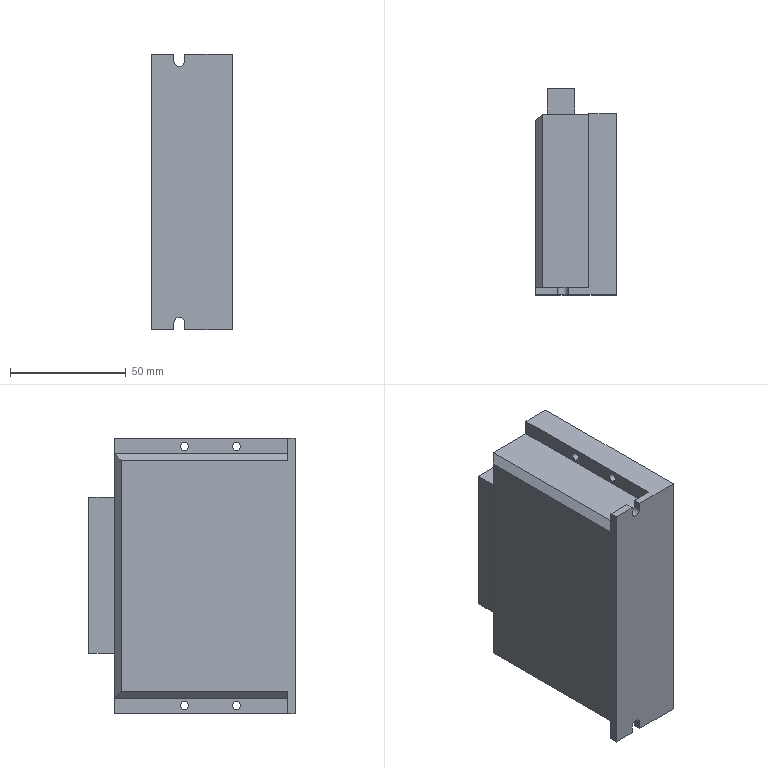Part | SolidWorks | features BaseBody 1 | 1 solid | 42 faces | box 35 x 89.2 x 119.2 mm | volume 310275 mm3 | plane 31 | cylinder 11 | commonest cylinder face diameters 3.5 x8 4.6 x3
STEP:
#1=CARTESIAN_POINT('',(17.5,25.3,54.25));
#2=VERTEX_POINT('',#1);
#3=CARTESIAN_POINT('',(5.5,25.3,54.25));
#4=VERTEX_POINT('',#3);
#5=CARTESIAN_POINT('',(17.501,25.3,54.25));
#6=DIRECTION('',(-1.,0.,0.));
#7=VECTOR('',#6,1000.);
#8=LINE('',#5,#7);
#9=EDGE_CURVE('',#2,#4,#8,.T.);
#10=ORIENTED_EDGE('',*,*,#9,.F.);
#11=CARTESIAN_POINT('',(17.5,25.3,57.75));
#12=VERTEX_POINT('',#11);
#13=CARTESIAN_POINT('',(17.5,25.3,56.));
#14=DIRECTION('',(1.,0.,0.));
#15=DIRECTION('',(0.,0.,1.));
#16=AXIS2_PLACEMENT_3D('',#13,#14,#15);
#17=CIRCLE('',#16,1.75);
#18=EDGE_CURVE('',#2,#12,#17,.T.);
#19=ORIENTED_EDGE('',*,*,#18,.T.);
#20=CARTESIAN_POINT('',(5.5,25.3,57.75));
#21=VERTEX_POINT('',#20);
#22=CARTESIAN_POINT('',(17.501,25.3,57.75));
#23=DIRECTION('',(-1.,0.,0.));
#24=VECTOR('',#23,1000.);
#25=LINE('',#22,#24);
#26=EDGE_CURVE('',#12,#21,#25,.T.);
#27=ORIENTED_EDGE('',*,*,#26,.T.);
#28=CARTESIAN_POINT('',(5.5,25.3,56.));
#29=DIRECTION('',(-1.,0.,0.));
#30=DIRECTION('',(0.,0.,-1.));
#31=AXIS2_PLACEMENT_3D('',#28,#29,#30);
#32=CIRCLE('',#31,1.75);
#33=EDGE_CURVE('',#21,#4,#32,.T.);
#34=ORIENTED_EDGE('',*,*,#33,.T.);
#35=EDGE_LOOP('',(#10,#19,#27,#34));
#36=FACE_OUTER_BOUND('',#35,.T.);
#37=CARTESIAN_POINT('',(17.501,25.3,56.));
#38=DIRECTION('',(-1.,0.,0.));
#39=DIRECTION('',(0.,0.,1.));
#40=AXIS2_PLACEMENT_3D('',#37,#38,#39);
#41=CYLINDRICAL_SURFACE('',#40,1.75);
#42=ADVANCED_FACE('',(#36),#41,.F.);
#43=CARTESIAN_POINT('',(17.5,47.8,54.25));
#44=VERTEX_POINT('',#43);
#45=CARTESIAN_POINT('',(5.5,47.8,54.25));
#46=VERTEX_POINT('',#45);
#47=CARTESIAN_POINT('',(17.501,47.8,54.25));
#48=DIRECTION('',(-1.,0.,0.));
#49=VECTOR('',#48,1000.);
#50=LINE('',#47,#49);
#51=EDGE_CURVE('',#44,#46,#50,.T.);
#52=ORIENTED_EDGE('',*,*,#51,.F.);
#53=CARTESIAN_POINT('',(17.5,47.8,57.75));
#54=VERTEX_POINT('',#53);
#55=CARTESIAN_POINT('',(17.5,47.8,56.));
#56=DIRECTION('',(1.,0.,0.));
#57=DIRECTION('',(0.,0.,1.));
#58=AXIS2_PLACEMENT_3D('',#55,#56,#57);
#59=CIRCLE('',#58,1.75);
#60=EDGE_CURVE('',#44,#54,#59,.T.);
#61=ORIENTED_EDGE('',*,*,#60,.T.);
#62=CARTESIAN_POINT('',(5.5,47.8,57.75));
#63=VERTEX_POINT('',#62);
#64=CARTESIAN_POINT('',(17.501,47.8,57.75));
#65=DIRECTION('',(-1.,0.,0.));
#66=VECTOR('',#65,1000.);
#67=LINE('',#64,#66);
#68=EDGE_CURVE('',#54,#63,#67,.T.);
#69=ORIENTED_EDGE('',*,*,#68,.T.);
#70=CARTESIAN_POINT('',(5.5,47.8,56.));
#71=DIRECTION('',(-1.,0.,0.));
#72=DIRECTION('',(0.,0.,-1.));
#73=AXIS2_PLACEMENT_3D('',#70,#71,#72);
#74=CIRCLE('',#73,1.75);
#75=EDGE_CURVE('',#63,#46,#74,.T.);
#76=ORIENTED_EDGE('',*,*,#75,.T.);
#77=EDGE_LOOP('',(#52,#61,#69,#76));
#78=FACE_OUTER_BOUND('',#77,.T.);
#79=CARTESIAN_POINT('',(17.501,47.8,56.));
#80=DIRECTION('',(-1.,0.,0.));
#81=DIRECTION('',(0.,0.,1.));
#82=AXIS2_PLACEMENT_3D('',#79,#80,#81);
#83=CYLINDRICAL_SURFACE('',#82,1.75);
#84=ADVANCED_FACE('',(#78),#83,.F.);
#85=CARTESIAN_POINT('',(17.5,47.8,-57.75));
#86=VERTEX_POINT('',#85);
#87=CARTESIAN_POINT('',(5.5,47.8,-57.75));
#88=VERTEX_POINT('',#87);
#89=CARTESIAN_POINT('',(17.501,47.8,-57.75));
#90=DIRECTION('',(-1.,0.,0.));
#91=VECTOR('',#90,1000.);
#92=LINE('',#89,#91);
#93=EDGE_CURVE('',#86,#88,#92,.T.);
#94=ORIENTED_EDGE('',*,*,#93,.F.);
#95=CARTESIAN_POINT('',(17.5,47.8,-54.25));
#96=VERTEX_POINT('',#95);
#97=CARTESIAN_POINT('',(17.5,47.8,-56.));
#98=DIRECTION('',(1.,0.,0.));
#99=DIRECTION('',(0.,0.,1.));
#100=AXIS2_PLACEMENT_3D('',#97,#98,#99);
#101=CIRCLE('',#100,1.75);
#102=EDGE_CURVE('',#86,#96,#101,.T.);
#103=ORIENTED_EDGE('',*,*,#102,.T.);
#104=CARTESIAN_POINT('',(5.5,47.8,-54.25));
#105=VERTEX_POINT('',#104);
#106=CARTESIAN_POINT('',(17.501,47.8,-54.25));
#107=DIRECTION('',(-1.,0.,0.));
#108=VECTOR('',#107,1000.);
#109=LINE('',#106,#108);
#110=EDGE_CURVE('',#96,#105,#109,.T.);
#111=ORIENTED_EDGE('',*,*,#110,.T.);
#112=CARTESIAN_POINT('',(5.5,47.8,-56.));
#113=DIRECTION('',(-1.,0.,0.));
#114=DIRECTION('',(0.,0.,1.));
#115=AXIS2_PLACEMENT_3D('',#112,#113,#114);
#116=CIRCLE('',#115,1.75);
#117=EDGE_CURVE('',#105,#88,#116,.T.);
#118=ORIENTED_EDGE('',*,*,#117,.T.);
#119=EDGE_LOOP('',(#94,#103,#111,#118));
#120=FACE_OUTER_BOUND('',#119,.T.);
#121=CARTESIAN_POINT('',(17.501,47.8,-56.));
#122=DIRECTION('',(-1.,0.,0.));
#123=DIRECTION('',(0.,0.,1.));
#124=AXIS2_PLACEMENT_3D('',#121,#122,#123);
#125=CYLINDRICAL_SURFACE('',#124,1.75);
#126=ADVANCED_FACE('',(#120),#125,.F.);
#127=CARTESIAN_POINT('',(17.5,25.3,-57.75));
#128=VERTEX_POINT('',#127);
#129=CARTESIAN_POINT('',(5.5,25.3,-57.75));
#130=VERTEX_POINT('',#129);
#131=CARTESIAN_POINT('',(17.501,25.3,-57.75));
#132=DIRECTION('',(-1.,0.,0.));
#133=VECTOR('',#132,1000.);
#134=LINE('',#131,#133);
#135=EDGE_CURVE('',#128,#130,#134,.T.);
#136=ORIENTED_EDGE('',*,*,#135,.F.);
#137=CARTESIAN_POINT('',(17.5,25.3,-54.25));
#138=VERTEX_POINT('',#137);
#139=CARTESIAN_POINT('',(17.5,25.3,-56.));
#140=DIRECTION('',(1.,0.,0.));
#141=DIRECTION('',(0.,0.,1.));
#142=AXIS2_PLACEMENT_3D('',#139,#140,#141);
#143=CIRCLE('',#142,1.75);
#144=EDGE_CURVE('',#128,#138,#143,.T.);
#145=ORIENTED_EDGE('',*,*,#144,.T.);
#146=CARTESIAN_POINT('',(5.5,25.3,-54.25));
#147=VERTEX_POINT('',#146);
#148=CARTESIAN_POINT('',(17.501,25.3,-54.25));
#149=DIRECTION('',(-1.,0.,0.));
#150=VECTOR('',#149,1000.);
#151=LINE('',#148,#150);
#152=EDGE_CURVE('',#138,#147,#151,.T.);
#153=ORIENTED_EDGE('',*,*,#152,.T.);
#154=CARTESIAN_POINT('',(5.5,25.3,-56.));
#155=DIRECTION('',(-1.,0.,0.));
#156=DIRECTION('',(0.,0.,1.));
#157=AXIS2_PLACEMENT_3D('',#154,#155,#156);
#158=CIRCLE('',#157,1.75);
#159=EDGE_CURVE('',#147,#130,#158,.T.);
#160=ORIENTED_EDGE('',*,*,#159,.T.);
#161=EDGE_LOOP('',(#136,#145,#153,#160));
#162=FACE_OUTER_BOUND('',#161,.T.);
#163=CARTESIAN_POINT('',(17.501,25.3,-56.));
#164=DIRECTION('',(-1.,0.,0.));
#165=DIRECTION('',(0.,0.,1.));
#166=AXIS2_PLACEMENT_3D('',#163,#164,#165);
#167=CYLINDRICAL_SURFACE('',#166,1.75);
#168=ADVANCED_FACE('',(#162),#167,.F.);
#169=CARTESIAN_POINT('',(-12.5,89.2,-33.5));
#170=VERTEX_POINT('',#169);
#171=CARTESIAN_POINT('',(-12.5,89.2,34.));
#172=VERTEX_POINT('',#171);
#173=CARTESIAN_POINT('',(-12.5,89.2,-33.5));
#174=DIRECTION('',(0.,0.,1.));
#175=VECTOR('',#174,1000.);
#176=LINE('',#173,#175);
#177=EDGE_CURVE('',#170,#172,#176,.T.);
#178=ORIENTED_EDGE('',*,*,#177,.T.);
#179=CARTESIAN_POINT('',(-0.5,89.2,34.));
#180=VERTEX_POINT('',#179);
#181=CARTESIAN_POINT('',(-12.5,89.2,34.));
#182=DIRECTION('',(1.,0.,0.));
#183=VECTOR('',#182,1000.);
#184=LINE('',#181,#183);
#185=EDGE_CURVE('',#172,#180,#184,.T.);
#186=ORIENTED_EDGE('',*,*,#185,.T.);
#187=CARTESIAN_POINT('',(-0.5,89.2,-33.5));
#188=VERTEX_POINT('',#187);
#189=CARTESIAN_POINT('',(-0.5,89.2,-33.5));
#190=DIRECTION('',(0.,0.,-1.));
#191=VECTOR('',#190,1000.);
#192=LINE('',#189,#191);
#193=EDGE_CURVE('',#180,#188,#192,.T.);
#194=ORIENTED_EDGE('',*,*,#193,.T.);
#195=CARTESIAN_POINT('',(-12.5,89.2,-33.5));
#196=DIRECTION('',(-1.,0.,0.));
#197=VECTOR('',#196,1000.);
#198=LINE('',#195,#197);
#199=EDGE_CURVE('',#188,#170,#198,.T.);
#200=ORIENTED_EDGE('',*,*,#199,.T.);
#201=EDGE_LOOP('',(#178,#186,#194,#200));
#202=FACE_OUTER_BOUND('',#201,.T.);
#203=CARTESIAN_POINT('',(0.,89.2,0.));
#204=DIRECTION('',(0.,1.,0.));
#205=DIRECTION('',(1.,0.,0.));
#206=AXIS2_PLACEMENT_3D('',#203,#204,#205);
#207=PLANE('',#206);
#208=ADVANCED_FACE('',(#202),#207,.T.);
#209=CARTESIAN_POINT('',(-0.5,78.2,-33.5));
#210=VERTEX_POINT('',#209);
#211=CARTESIAN_POINT('',(-12.5,78.2,-33.5));
#212=VERTEX_POINT('',#211);
#213=CARTESIAN_POINT('',(-12.5,78.2,-33.5));
#214=DIRECTION('',(-1.,0.,0.));
#215=VECTOR('',#214,1000.);
#216=LINE('',#213,#215);
#217=EDGE_CURVE('',#210,#212,#216,.T.);
#218=ORIENTED_EDGE('',*,*,#217,.T.);
#219=CARTESIAN_POINT('',(-12.5,89.2,-33.5));
#220=DIRECTION('',(0.,-1.,0.));
#221=VECTOR('',#220,1000.);
#222=LINE('',#219,#221);
#223=EDGE_CURVE('',#170,#212,#222,.T.);
#224=ORIENTED_EDGE('',*,*,#223,.F.);
#225=ORIENTED_EDGE('',*,*,#199,.F.);
#226=CARTESIAN_POINT('',(-0.5,89.2,-33.5));
#227=DIRECTION('',(0.,-1.,0.));
#228=VECTOR('',#227,1000.);
#229=LINE('',#226,#228);
#230=EDGE_CURVE('',#188,#210,#229,.T.);
#231=ORIENTED_EDGE('',*,*,#230,.T.);
#232=EDGE_LOOP('',(#218,#224,#225,#231));
#233=FACE_OUTER_BOUND('',#232,.T.);
#234=CARTESIAN_POINT('',(-12.5,89.2,-33.5));
#235=DIRECTION('',(0.,0.,1.));
#236=DIRECTION('',(1.,0.,0.));
#237=AXIS2_PLACEMENT_3D('',#234,#235,#236);
#238=PLANE('',#237);
#239=ADVANCED_FACE('',(#233),#238,.F.);
#240=CARTESIAN_POINT('',(-0.5,78.2,34.));
#241=VERTEX_POINT('',#240);
#242=CARTESIAN_POINT('',(-0.5,78.2,-33.5));
#243=DIRECTION('',(0.,0.,-1.));
#244=VECTOR('',#243,1000.);
#245=LINE('',#242,#244);
#246=EDGE_CURVE('',#241,#210,#245,.T.);
#247=ORIENTED_EDGE('',*,*,#246,.T.);
#248=ORIENTED_EDGE('',*,*,#230,.F.);
#249=ORIENTED_EDGE('',*,*,#193,.F.);
#250=CARTESIAN_POINT('',(-0.5,89.2,34.));
#251=DIRECTION('',(0.,-1.,0.));
#252=VECTOR('',#251,1000.);
#253=LINE('',#250,#252);
#254=EDGE_CURVE('',#180,#241,#253,.T.);
#255=ORIENTED_EDGE('',*,*,#254,.T.);
#256=EDGE_LOOP('',(#247,#248,#249,#255));
#257=FACE_OUTER_BOUND('',#256,.T.);
#258=CARTESIAN_POINT('',(-0.5,89.2,-33.5));
#259=DIRECTION('',(-1.,0.,0.));
#260=DIRECTION('',(0.,1.,0.));
#261=AXIS2_PLACEMENT_3D('',#258,#259,#260);
#262=PLANE('',#261);
#263=ADVANCED_FACE('',(#257),#262,.F.);
#264=CARTESIAN_POINT('',(-12.5,78.2,34.));
#265=VERTEX_POINT('',#264);
#266=CARTESIAN_POINT('',(-12.5,78.2,34.));
#267=DIRECTION('',(1.,0.,0.));
#268=VECTOR('',#267,1000.);
#269=LINE('',#266,#268);
#270=EDGE_CURVE('',#265,#241,#269,.T.);
#271=ORIENTED_EDGE('',*,*,#270,.T.);
#272=ORIENTED_EDGE('',*,*,#254,.F.);
#273=ORIENTED_EDGE('',*,*,#185,.F.);
#274=CARTESIAN_POINT('',(-12.5,89.2,34.));
#275=DIRECTION('',(0.,-1.,0.));
#276=VECTOR('',#275,1000.);
#277=LINE('',#274,#276);
#278=EDGE_CURVE('',#172,#265,#277,.T.);
#279=ORIENTED_EDGE('',*,*,#278,.T.);
#280=EDGE_LOOP('',(#271,#272,#273,#279));
#281=FACE_OUTER_BOUND('',#280,.T.);
#282=CARTESIAN_POINT('',(-12.5,89.2,34.));
#283=DIRECTION('',(0.,0.,-1.));
#284=DIRECTION('',(0.,-1.,0.));
#285=AXIS2_PLACEMENT_3D('',#282,#283,#284);
#286=PLANE('',#285);
#287=ADVANCED_FACE('',(#281),#286,.F.);
#288=CARTESIAN_POINT('',(-12.5,78.2,-33.5));
#289=DIRECTION('',(0.,0.,1.));
#290=VECTOR('',#289,1000.);
#291=LINE('',#288,#290);
#292=EDGE_CURVE('',#212,#265,#291,.T.);
#293=ORIENTED_EDGE('',*,*,#292,.T.);
#294=ORIENTED_EDGE('',*,*,#278,.F.);
#295=ORIENTED_EDGE('',*,*,#177,.F.);
#296=ORIENTED_EDGE('',*,*,#223,.T.);
#297=EDGE_LOOP('',(#293,#294,#295,#296));
#298=FACE_OUTER_BOUND('',#297,.T.);
#299=CARTESIAN_POINT('',(-12.5,89.2,-33.5));
#300=DIRECTION('',(1.,0.,0.));
#301=DIRECTION('',(0.,0.,-1.));
#302=AXIS2_PLACEMENT_3D('',#299,#300,#301);
#303=PLANE('',#302);
#304=ADVANCED_FACE('',(#298),#303,.F.);
#305=CARTESIAN_POINT('',(-1.5,50.5,-52.));
#306=VERTEX_POINT('',#305);
#307=CARTESIAN_POINT('',(-1.5,19.2,-52.));
#308=VERTEX_POINT('',#307);
#309=CARTESIAN_POINT('',(-1.5,50.5,-52.));
#310=DIRECTION('',(0.,-1.,0.));
#311=VECTOR('',#310,1000.);
#312=LINE('',#309,#311);
#313=EDGE_CURVE('',#306,#308,#312,.T.);
#314=ORIENTED_EDGE('',*,*,#313,.T.);
#315=CARTESIAN_POINT('',(-13.5,19.2,-52.));
#316=VERTEX_POINT('',#315);
#317=CARTESIAN_POINT('',(-1.5,19.2,-52.));
#318=DIRECTION('',(-1.,0.,0.));
#319=VECTOR('',#318,1000.);
#320=LINE('',#317,#319);
#321=EDGE_CURVE('',#308,#316,#320,.T.);
#322=ORIENTED_EDGE('',*,*,#321,.T.);
#323=CARTESIAN_POINT('',(-13.5,50.5,-52.));
#324=VERTEX_POINT('',#323);
#325=CARTESIAN_POINT('',(-13.5,50.5,-52.));
#326=DIRECTION('',(0.,1.,0.));
#327=VECTOR('',#326,1000.);
#328=LINE('',#325,#327);
#329=EDGE_CURVE('',#316,#324,#328,.T.);
#330=ORIENTED_EDGE('',*,*,#329,.T.);
#331=CARTESIAN_POINT('',(-1.5,50.5,-52.));
#332=DIRECTION('',(1.,0.,0.));
#333=VECTOR('',#332,1000.);
#334=LINE('',#331,#333);
#335=EDGE_CURVE('',#324,#306,#334,.T.);
#336=ORIENTED_EDGE('',*,*,#335,.T.);
#337=EDGE_LOOP('',(#314,#322,#330,#336));
#338=FACE_OUTER_BOUND('',#337,.T.);
#339=CARTESIAN_POINT('',(0.,0.,-52.));
#340=DIRECTION('',(0.,0.,-1.));
#341=DIRECTION('',(0.,-1.,0.));
#342=AXIS2_PLACEMENT_3D('',#339,#340,#341);
#343=PLANE('',#342);
#344=ADVANCED_FACE('',(#338),#343,.T.);
#345=CARTESIAN_POINT('',(-1.5,19.2,-53.));
#346=VERTEX_POINT('',#345);
#347=CARTESIAN_POINT('',(-13.5,19.2,-53.));
#348=VERTEX_POINT('',#347);
#349=CARTESIAN_POINT('',(-1.5,19.2,-53.));
#350=DIRECTION('',(-1.,0.,0.));
#351=VECTOR('',#350,1000.);
#352=LINE('',#349,#351);
#353=EDGE_CURVE('',#346,#348,#352,.T.);
#354=ORIENTED_EDGE('',*,*,#353,.T.);
#355=CARTESIAN_POINT('',(-13.5,19.2,-52.));
#356=DIRECTION('',(0.,0.,-1.));
#357=VECTOR('',#356,1000.);
#358=LINE('',#355,#357);
#359=EDGE_CURVE('',#316,#348,#358,.T.);
#360=ORIENTED_EDGE('',*,*,#359,.F.);
#361=ORIENTED_EDGE('',*,*,#321,.F.);
#362=CARTESIAN_POINT('',(-1.5,19.2,-52.));
#363=DIRECTION('',(0.,0.,-1.));
#364=VECTOR('',#363,1000.);
#365=LINE('',#362,#364);
#366=EDGE_CURVE('',#308,#346,#365,.T.);
#367=ORIENTED_EDGE('',*,*,#366,.T.);
#368=EDGE_LOOP('',(#354,#360,#361,#367));
#369=FACE_OUTER_BOUND('',#368,.T.);
#370=CARTESIAN_POINT('',(-1.5,19.2,-52.));
#371=DIRECTION('',(0.,-1.,0.));
#372=DIRECTION('',(0.,0.,-1.));
#373=AXIS2_PLACEMENT_3D('',#370,#371,#372);
#374=PLANE('',#373);
#375=ADVANCED_FACE('',(#369),#374,.F.);
#376=CARTESIAN_POINT('',(-13.5,50.5,-53.));
#377=VERTEX_POINT('',#376);
#378=CARTESIAN_POINT('',(-13.5,50.5,-53.));
#379=DIRECTION('',(0.,1.,0.));
#380=VECTOR('',#379,1000.);
#381=LINE('',#378,#380);
#382=EDGE_CURVE('',#348,#377,#381,.T.);
#383=ORIENTED_EDGE('',*,*,#382,.T.);
#384=CARTESIAN_POINT('',(-13.5,50.5,-52.));
#385=DIRECTION('',(0.,0.,-1.));
#386=VECTOR('',#385,1000.);
#387=LINE('',#384,#386);
#388=EDGE_CURVE('',#324,#377,#387,.T.);
#389=ORIENTED_EDGE('',*,*,#388,.F.);
#390=ORIENTED_EDGE('',*,*,#329,.F.);
#391=ORIENTED_EDGE('',*,*,#359,.T.);
#392=EDGE_LOOP('',(#383,#389,#390,#391));
#393=FACE_OUTER_BOUND('',#392,.T.);
#394=CARTESIAN_POINT('',(-13.5,50.5,-52.));
#395=DIRECTION('',(-1.,0.,0.));
#396=DIRECTION('',(0.,1.,0.));
#397=AXIS2_PLACEMENT_3D('',#394,#395,#396);
#398=PLANE('',#397);
#399=ADVANCED_FACE('',(#393),#398,.F.);
#400=CARTESIAN_POINT('',(-1.5,50.5,-53.));
#401=VERTEX_POINT('',#400);
#402=CARTESIAN_POINT('',(-1.5,50.5,-53.));
#403=DIRECTION('',(1.,0.,0.));
#404=VECTOR('',#403,1000.);
#405=LINE('',#402,#404);
#406=EDGE_CURVE('',#377,#401,#405,.T.);
#407=ORIENTED_EDGE('',*,*,#406,.T.);
#408=CARTESIAN_POINT('',(-1.5,50.5,-52.));
#409=DIRECTION('',(0.,0.,-1.));
#410=VECTOR('',#409,1000.);
#411=LINE('',#408,#410);
#412=EDGE_CURVE('',#306,#401,#411,.T.);
#413=ORIENTED_EDGE('',*,*,#412,.F.);
#414=ORIENTED_EDGE('',*,*,#335,.F.);
#415=ORIENTED_EDGE('',*,*,#388,.T.);
#416=EDGE_LOOP('',(#407,#413,#414,#415));
#417=FACE_OUTER_BOUND('',#416,.T.);
#418=CARTESIAN_POINT('',(-1.5,50.5,-52.));
#419=DIRECTION('',(0.,1.,0.));
#420=DIRECTION('',(1.,0.,0.));
#421=AXIS2_PLACEMENT_3D('',#418,#419,#420);
#422=PLANE('',#421);
#423=ADVANCED_FACE('',(#417),#422,.F.);
#424=CARTESIAN_POINT('',(-1.5,50.5,-53.));
#425=DIRECTION('',(0.,-1.,0.));
#426=VECTOR('',#425,1000.);
#427=LINE('',#424,#426);
#428=EDGE_CURVE('',#401,#346,#427,.T.);
#429=ORIENTED_EDGE('',*,*,#428,.T.);
#430=ORIENTED_EDGE('',*,*,#366,.F.);
#431=ORIENTED_EDGE('',*,*,#313,.F.);
#432=ORIENTED_EDGE('',*,*,#412,.T.);
#433=EDGE_LOOP('',(#429,#430,#431,#432));
#434=FACE_OUTER_BOUND('',#433,.T.);
#435=CARTESIAN_POINT('',(-1.5,50.5,-52.));
#436=DIRECTION('',(1.,0.,0.));
#437=DIRECTION('',(0.,-1.,0.));
#438=AXIS2_PLACEMENT_3D('',#435,#436,#437);
#439=PLANE('',#438);
#440=ADVANCED_FACE('',(#434),#439,.F.);
#441=CARTESIAN_POINT('',(-3.2,0.,-59.6));
#442=VERTEX_POINT('',#441);
#443=CARTESIAN_POINT('',(-3.2,0.,-56.5));
#444=VERTEX_POINT('',#443);
#445=CARTESIAN_POINT('',(-3.2,0.,-59.6));
#446=DIRECTION('',(0.,0.,1.));
#447=VECTOR('',#446,1000.);
#448=LINE('',#445,#447);
#449=EDGE_CURVE('',#442,#444,#448,.T.);
#450=ORIENTED_EDGE('',*,*,#449,.T.);
#451=CARTESIAN_POINT('',(-3.2,3.2,-56.5));
#452=VERTEX_POINT('',#451);
#453=CARTESIAN_POINT('',(-3.2,-0.001,-56.5));
#454=DIRECTION('',(0.,1.,0.));
#455=VECTOR('',#454,1000.);
#456=LINE('',#453,#455);
#457=EDGE_CURVE('',#444,#452,#456,.T.);
#458=ORIENTED_EDGE('',*,*,#457,.T.);
#459=CARTESIAN_POINT('',(-3.2,3.2,-59.6));
#460=VERTEX_POINT('',#459);
#461=CARTESIAN_POINT('',(-3.2,3.2,-59.6));
#462=DIRECTION('',(0.,0.,-1.));
#463=VECTOR('',#462,1000.);
#464=LINE('',#461,#463);
#465=EDGE_CURVE('',#452,#460,#464,.T.);
#466=ORIENTED_EDGE('',*,*,#465,.T.);
#467=CARTESIAN_POINT('',(-3.2,-0.001,-59.6));
#468=DIRECTION('',(0.,1.,0.));
#469=VECTOR('',#468,1000.);
#470=LINE('',#467,#469);
#471=EDGE_CURVE('',#442,#460,#470,.T.);
#472=ORIENTED_EDGE('',*,*,#471,.F.);
#473=EDGE_LOOP('',(#450,#458,#466,#472));
#474=FACE_OUTER_BOUND('',#473,.T.);
#475=CARTESIAN_POINT('',(-3.2,-0.001,-59.6));
#476=DIRECTION('',(1.,0.,0.));
#477=DIRECTION('',(0.,0.,-1.));
#478=AXIS2_PLACEMENT_3D('',#475,#476,#477);
#479=PLANE('',#478);
#480=ADVANCED_FACE('',(#474),#479,.F.);
#481=CARTESIAN_POINT('',(-7.8,0.,-56.5));
#482=VERTEX_POINT('',#481);
#483=CARTESIAN_POINT('',(-7.8,0.,-59.6));
#484=VERTEX_POINT('',#483);
#485=CARTESIAN_POINT('',(-7.8,0.,-56.5));
#486=DIRECTION('',(0.,0.,-1.));
#487=VECTOR('',#486,1000.);
#488=LINE('',#485,#487);
#489=EDGE_CURVE('',#482,#484,#488,.T.);
#490=ORIENTED_EDGE('',*,*,#489,.T.);
#491=CARTESIAN_POINT('',(-7.8,3.2,-59.6));
#492=VERTEX_POINT('',#491);
#493=CARTESIAN_POINT('',(-7.8,-0.001,-59.6));
#494=DIRECTION('',(0.,1.,0.));
#495=VECTOR('',#494,1000.);
#496=LINE('',#493,#495);
#497=EDGE_CURVE('',#484,#492,#496,.T.);
#498=ORIENTED_EDGE('',*,*,#497,.T.);
#499=CARTESIAN_POINT('',(-7.8,3.2,-56.5));
#500=VERTEX_POINT('',#499);
#501=CARTESIAN_POINT('',(-7.8,3.2,-56.5));
#502=DIRECTION('',(0.,0.,1.));
#503=VECTOR('',#502,1000.);
#504=LINE('',#501,#503);
#505=EDGE_CURVE('',#492,#500,#504,.T.);
#506=ORIENTED_EDGE('',*,*,#505,.T.);
#507=CARTESIAN_POINT('',(-7.8,-0.001,-56.5));
#508=DIRECTION('',(0.,1.,0.));
#509=VECTOR('',#508,1000.);
#510=LINE('',#507,#509);
#511=EDGE_CURVE('',#482,#500,#510,.T.);
#512=ORIENTED_EDGE('',*,*,#511,.F.);
#513=EDGE_LOOP('',(#490,#498,#506,#512));
#514=FACE_OUTER_BOUND('',#513,.T.);
#515=CARTESIAN_POINT('',(-7.8,-0.001,-56.5));
#516=DIRECTION('',(-1.,0.,0.));
#517=DIRECTION('',(0.,0.,1.));
#518=AXIS2_PLACEMENT_3D('',#515,#516,#517);
#519=PLANE('',#518);
#520=ADVANCED_FACE('',(#514),#519,.F.);
#521=CARTESIAN_POINT('',(-5.5,0.,-54.2));
#522=VERTEX_POINT('',#521);
#523=CARTESIAN_POINT('',(-5.5,3.2,-54.2));
#524=VERTEX_POINT('',#523);
#525=CARTESIAN_POINT('',(-5.5,-0.001,-54.2));
#526=DIRECTION('',(0.,1.,0.));
#527=VECTOR('',#526,1000.);
#528=LINE('',#525,#527);
#529=EDGE_CURVE('',#522,#524,#528,.T.);
#530=ORIENTED_EDGE('',*,*,#529,.F.);
#531=CARTESIAN_POINT('',(-5.5,0.,-56.5));
#532=DIRECTION('',(0.,-1.,0.));
#533=DIRECTION('',(0.,0.,1.));
#534=AXIS2_PLACEMENT_3D('',#531,#532,#533);
#535=CIRCLE('',#534,2.3);
#536=EDGE_CURVE('',#522,#482,#535,.T.);
#537=ORIENTED_EDGE('',*,*,#536,.T.);
#538=ORIENTED_EDGE('',*,*,#511,.T.);
#539=CARTESIAN_POINT('',(-5.5,3.2,-56.5));
#540=DIRECTION('',(0.,1.,0.));
#541=DIRECTION('',(0.,0.,1.));
#542=AXIS2_PLACEMENT_3D('',#539,#540,#541);
#543=CIRCLE('',#542,2.3);
#544=EDGE_CURVE('',#500,#524,#543,.T.);
#545=ORIENTED_EDGE('',*,*,#544,.T.);
#546=EDGE_LOOP('',(#530,#537,#538,#545));
#547=FACE_OUTER_BOUND('',#546,.T.);
#548=CARTESIAN_POINT('',(-5.5,-0.001,-56.5));
#549=DIRECTION('',(0.,1.,0.));
#550=DIRECTION('',(0.,0.,1.));
#551=AXIS2_PLACEMENT_3D('',#548,#549,#550);
#552=CYLINDRICAL_SURFACE('',#551,2.3);
#553=ADVANCED_FACE('',(#547),#552,.F.);
#554=CARTESIAN_POINT('',(-7.8,0.,59.6));
#555=VERTEX_POINT('',#554);
#556=CARTESIAN_POINT('',(-7.8,0.,56.5));
#557=VERTEX_POINT('',#556);
#558=CARTESIAN_POINT('',(-7.8,0.,56.5));
#559=DIRECTION('',(0.,0.,-1.));
#560=VECTOR('',#559,1000.);
#561=LINE('',#558,#560);
#562=EDGE_CURVE('',#555,#557,#561,.T.);
#563=ORIENTED_EDGE('',*,*,#562,.T.);
#564=CARTESIAN_POINT('',(-7.8,3.2,56.5));
#565=VERTEX_POINT('',#564);
#566=CARTESIAN_POINT('',(-7.8,-0.001,56.5));
#567=DIRECTION('',(0.,1.,0.));
#568=VECTOR('',#567,1000.);
#569=LINE('',#566,#568);
#570=EDGE_CURVE('',#557,#565,#569,.T.);
#571=ORIENTED_EDGE('',*,*,#570,.T.);
#572=CARTESIAN_POINT('',(-7.8,3.2,59.6));
#573=VERTEX_POINT('',#572);
#574=CARTESIAN_POINT('',(-7.8,3.2,56.5));
#575=DIRECTION('',(0.,0.,1.));
#576=VECTOR('',#575,1000.);
#577=LINE('',#574,#576);
#578=EDGE_CURVE('',#565,#573,#577,.T.);
#579=ORIENTED_EDGE('',*,*,#578,.T.);
#580=CARTESIAN_POINT('',(-7.8,-0.001,59.6));
#581=DIRECTION('',(0.,1.,0.));
#582=VECTOR('',#581,1000.);
#583=LINE('',#580,#582);
#584=EDGE_CURVE('',#555,#573,#583,.T.);
#585=ORIENTED_EDGE('',*,*,#584,.F.);
#586=EDGE_LOOP('',(#563,#571,#579,#585));
#587=FACE_OUTER_BOUND('',#586,.T.);
#588=CARTESIAN_POINT('',(-7.8,-0.001,56.5));
#589=DIRECTION('',(-1.,0.,0.));
#590=DIRECTION('',(0.,0.,1.));
#591=AXIS2_PLACEMENT_3D('',#588,#589,#590);
#592=PLANE('',#591);
#593=ADVANCED_FACE('',(#587),#592,.F.);
#594=CARTESIAN_POINT('',(-3.2,0.,56.5));
#595=VERTEX_POINT('',#594);
#596=CARTESIAN_POINT('',(-3.2,0.,59.6));
#597=VERTEX_POINT('',#596);
#598=CARTESIAN_POINT('',(-3.2,0.,59.6));
#599=DIRECTION('',(0.,0.,1.));
#600=VECTOR('',#599,1000.);
#601=LINE('',#598,#600);
#602=EDGE_CURVE('',#595,#597,#601,.T.);
#603=ORIENTED_EDGE('',*,*,#602,.T.);
#604=CARTESIAN_POINT('',(-3.2,3.2,59.6));
#605=VERTEX_POINT('',#604);
#606=CARTESIAN_POINT('',(-3.2,-0.001,59.6));
#607=DIRECTION('',(0.,1.,0.));
#608=VECTOR('',#607,1000.);
#609=LINE('',#606,#608);
#610=EDGE_CURVE('',#597,#605,#609,.T.);
#611=ORIENTED_EDGE('',*,*,#610,.T.);
#612=CARTESIAN_POINT('',(-3.2,3.2,56.5));
#613=VERTEX_POINT('',#612);
#614=CARTESIAN_POINT('',(-3.2,3.2,59.6));
#615=DIRECTION('',(0.,0.,-1.));
#616=VECTOR('',#615,1000.);
#617=LINE('',#614,#616);
#618=EDGE_CURVE('',#605,#613,#617,.T.);
#619=ORIENTED_EDGE('',*,*,#618,.T.);
#620=CARTESIAN_POINT('',(-3.2,-0.001,56.5));
#621=DIRECTION('',(0.,1.,0.));
#622=VECTOR('',#621,1000.);
#623=LINE('',#620,#622);
#624=EDGE_CURVE('',#595,#613,#623,.T.);
#625=ORIENTED_EDGE('',*,*,#624,.F.);
#626=EDGE_LOOP('',(#603,#611,#619,#625));
#627=FACE_OUTER_BOUND('',#626,.T.);
#628=CARTESIAN_POINT('',(-3.2,-0.001,59.6));
#629=DIRECTION('',(1.,0.,0.));
#630=DIRECTION('',(0.,0.,1.));
#631=AXIS2_PLACEMENT_3D('',#628,#629,#630);
#632=PLANE('',#631);
#633=ADVANCED_FACE('',(#627),#632,.F.);
#634=CARTESIAN_POINT('',(-5.5,0.,56.5));
#635=DIRECTION('',(0.,-1.,0.));
#636=DIRECTION('',(0.,0.,1.));
#637=AXIS2_PLACEMENT_3D('',#634,#635,#636);
#638=CIRCLE('',#637,2.3);
#639=EDGE_CURVE('',#557,#595,#638,.T.);
#640=ORIENTED_EDGE('',*,*,#639,.T.);
#641=ORIENTED_EDGE('',*,*,#624,.T.);
#642=CARTESIAN_POINT('',(-5.5,3.2,56.5));
#643=DIRECTION('',(0.,1.,0.));
#644=DIRECTION('',(0.,0.,-1.));
#645=AXIS2_PLACEMENT_3D('',#642,#643,#644);
#646=CIRCLE('',#645,2.3);
#647=EDGE_CURVE('',#613,#565,#646,.T.);
#648=ORIENTED_EDGE('',*,*,#647,.T.);
#649=ORIENTED_EDGE('',*,*,#570,.F.);
#650=EDGE_LOOP('',(#640,#641,#648,#649));
#651=FACE_OUTER_BOUND('',#650,.T.);
#652=CARTESIAN_POINT('',(-5.5,-0.001,56.5));
#653=DIRECTION('',(0.,1.,0.));
#654=DIRECTION('',(0.,0.,1.));
#655=AXIS2_PLACEMENT_3D('',#652,#653,#654);
#656=CYLINDRICAL_SURFACE('',#655,2.3);
#657=ADVANCED_FACE('',(#651),#656,.F.);
#658=CARTESIAN_POINT('',(-14.5,78.2,53.));
#659=VERTEX_POINT('',#658);
#660=CARTESIAN_POINT('',(-17.5,75.2,50.));
#661=VERTEX_POINT('',#660);
#662=CARTESIAN_POINT('',(-32.167,60.533,35.333));
#663=DIRECTION('',(-0.5774,-0.5774,-0.5774));
#664=VECTOR('',#663,1000.);
#665=LINE('',#662,#664);
#666=EDGE_CURVE('',#659,#661,#665,.T.);
#667=ORIENTED_EDGE('',*,*,#666,.T.);
#668=CARTESIAN_POINT('',(-17.5,3.2,50.));
#669=VERTEX_POINT('',#668);
#670=CARTESIAN_POINT('',(-17.5,3.2,50.));
#671=DIRECTION('',(0.,1.,0.));
#672=VECTOR('',#671,1000.);
#673=LINE('',#670,#672);
#674=EDGE_CURVE('',#669,#661,#673,.T.);
#675=ORIENTED_EDGE('',*,*,#674,.F.);
#676=CARTESIAN_POINT('',(-14.5,3.2,53.));
#677=VERTEX_POINT('',#676);
#678=CARTESIAN_POINT('',(-14.5,3.2,53.));
#679=DIRECTION('',(-0.7071,0.,-0.7071));
#680=VECTOR('',#679,1000.);
#681=LINE('',#678,#680);
#682=EDGE_CURVE('',#677,#669,#681,.T.);
#683=ORIENTED_EDGE('',*,*,#682,.F.);
#684=CARTESIAN_POINT('',(-14.5,3.2,53.));
#685=DIRECTION('',(0.,-1.,0.));
#686=VECTOR('',#685,1000.);
#687=LINE('',#684,#686);
#688=EDGE_CURVE('',#659,#677,#687,.T.);
#689=ORIENTED_EDGE('',*,*,#688,.F.);
#690=EDGE_LOOP('',(#667,#675,#683,#689));
#691=FACE_OUTER_BOUND('',#690,.T.);
#692=CARTESIAN_POINT('',(-14.5,3.2,53.));
#693=DIRECTION('',(0.7071,0.,-0.7071));
#694=DIRECTION('',(0.,-1.,0.));
#695=AXIS2_PLACEMENT_3D('',#692,#693,#694);
#696=PLANE('',#695);
#697=ADVANCED_FACE('',(#691),#696,.F.);
#698=CARTESIAN_POINT('',(-14.5,78.2,-53.));
#699=VERTEX_POINT('',#698);
#700=CARTESIAN_POINT('',(-17.5,75.2,-50.));
#701=VERTEX_POINT('',#700);
#702=CARTESIAN_POINT('',(-39.5,53.2,-28.));
#703=DIRECTION('',(-0.5774,-0.5774,0.5774));
#704=VECTOR('',#703,1000.);
#705=LINE('',#702,#704);
#706=EDGE_CURVE('',#699,#701,#705,.T.);
#707=ORIENTED_EDGE('',*,*,#706,.T.);
#708=CARTESIAN_POINT('',(-17.5,75.2,-59.6));
#709=DIRECTION('',(0.,0.,-1.));
#710=VECTOR('',#709,1000.);
#711=LINE('',#708,#710);
#712=EDGE_CURVE('',#661,#701,#711,.T.);
#713=ORIENTED_EDGE('',*,*,#712,.F.);
#714=ORIENTED_EDGE('',*,*,#666,.F.);
#715=CARTESIAN_POINT('',(-14.5,78.2,0.));
#716=DIRECTION('',(0.,0.,1.));
#717=VECTOR('',#716,1000.);
#718=LINE('',#715,#717);
#719=EDGE_CURVE('',#699,#659,#718,.T.);
#720=ORIENTED_EDGE('',*,*,#719,.F.);
#721=EDGE_LOOP('',(#707,#713,#714,#720));
#722=FACE_OUTER_BOUND('',#721,.T.);
#723=CARTESIAN_POINT('',(-14.5,78.2,0.));
#724=DIRECTION('',(0.7071,-0.7071,0.));
#725=DIRECTION('',(0.,0.,-1.));
#726=AXIS2_PLACEMENT_3D('',#723,#724,#725);
#727=PLANE('',#726);
#728=ADVANCED_FACE('',(#722),#727,.F.);
#729=CARTESIAN_POINT('',(-17.5,3.2,-50.));
#730=VERTEX_POINT('',#729);
#731=CARTESIAN_POINT('',(-14.5,3.2,-53.));
#732=VERTEX_POINT('',#731);
#733=CARTESIAN_POINT('',(-14.5,3.2,-53.));
#734=DIRECTION('',(0.7071,0.,-0.7071));
#735=VECTOR('',#734,1000.);
#736=LINE('',#733,#735);
#737=EDGE_CURVE('',#730,#732,#736,.T.);
#738=ORIENTED_EDGE('',*,*,#737,.F.);
#739=CARTESIAN_POINT('',(-17.5,3.2,-50.));
#740=DIRECTION('',(0.,-1.,0.));
#741=VECTOR('',#740,1000.);
#742=LINE('',#739,#741);
#743=EDGE_CURVE('',#701,#730,#742,.T.);
#744=ORIENTED_EDGE('',*,*,#743,.F.);
#745=ORIENTED_EDGE('',*,*,#706,.F.);
#746=CARTESIAN_POINT('',(-14.5,3.2,-53.));
#747=DIRECTION('',(0.,1.,0.));
#748=VECTOR('',#747,1000.);
#749=LINE('',#746,#748);
#750=EDGE_CURVE('',#732,#699,#749,.T.);
#751=ORIENTED_EDGE('',*,*,#750,.F.);
#752=EDGE_LOOP('',(#738,#744,#745,#751));
#753=FACE_OUTER_BOUND('',#752,.T.);
#754=CARTESIAN_POINT('',(-14.5,3.2,-53.));
#755=DIRECTION('',(0.7071,0.,0.7071));
#756=DIRECTION('',(0.,-1.,0.));
#757=AXIS2_PLACEMENT_3D('',#754,#755,#756);
#758=PLANE('',#757);
#759=ADVANCED_FACE('',(#753),#758,.F.);
#760=ORIENTED_EDGE('',*,*,#353,.F.);
#761=ORIENTED_EDGE('',*,*,#428,.F.);
#762=ORIENTED_EDGE('',*,*,#406,.F.);
#763=ORIENTED_EDGE('',*,*,#382,.F.);
#764=EDGE_LOOP('',(#760,#761,#762,#763));
#765=FACE_BOUND('',#764,.T.);
#766=CARTESIAN_POINT('',(5.5,3.2,-53.));
#767=VERTEX_POINT('',#766);
#768=CARTESIAN_POINT('',(-147.35,3.2,-53.));
#769=DIRECTION('',(1.,0.,0.));
#770=VECTOR('',#769,1000.);
#771=LINE('',#768,#770);
#772=EDGE_CURVE('',#732,#767,#771,.T.);
#773=ORIENTED_EDGE('',*,*,#772,.F.);
#774=ORIENTED_EDGE('',*,*,#750,.T.);
#775=CARTESIAN_POINT('',(5.5,78.2,-53.));
#776=VERTEX_POINT('',#775);
#777=CARTESIAN_POINT('',(-147.35,78.2,-53.));
#778=DIRECTION('',(1.,0.,0.));
#779=VECTOR('',#778,1000.);
#780=LINE('',#777,#779);
#781=EDGE_CURVE('',#699,#776,#780,.T.);
#782=ORIENTED_EDGE('',*,*,#781,.T.);
#783=CARTESIAN_POINT('',(5.5,3.2,-53.));
#784=DIRECTION('',(0.,-1.,0.));
#785=VECTOR('',#784,1000.);
#786=LINE('',#783,#785);
#787=EDGE_CURVE('',#776,#767,#786,.T.);
#788=ORIENTED_EDGE('',*,*,#787,.T.);
#789=EDGE_LOOP('',(#773,#774,#782,#788));
#790=FACE_OUTER_BOUND('',#789,.T.);
#791=CARTESIAN_POINT('',(-147.35,3.2,-53.));
#792=DIRECTION('',(0.,0.,1.));
#793=DIRECTION('',(1.,0.,0.));
#794=AXIS2_PLACEMENT_3D('',#791,#792,#793);
#795=PLANE('',#794);
#796=ADVANCED_FACE('',(#765,#790),#795,.F.);
#797=CARTESIAN_POINT('',(5.5,78.2,53.));
#798=VERTEX_POINT('',#797);
#799=CARTESIAN_POINT('',(-147.35,78.2,53.));
#800=DIRECTION('',(1.,0.,0.));
#801=VECTOR('',#800,1000.);
#802=LINE('',#799,#801);
#803=EDGE_CURVE('',#659,#798,#802,.T.);
#804=ORIENTED_EDGE('',*,*,#803,.F.);
#805=ORIENTED_EDGE('',*,*,#688,.T.);
#806=CARTESIAN_POINT('',(5.5,3.2,53.));
#807=VERTEX_POINT('',#806);
#808=CARTESIAN_POINT('',(-147.35,3.2,53.));
#809=DIRECTION('',(1.,0.,0.));
#810=VECTOR('',#809,1000.);
#811=LINE('',#808,#810);
#812=EDGE_CURVE('',#677,#807,#811,.T.);
#813=ORIENTED_EDGE('',*,*,#812,.T.);
#814=CARTESIAN_POINT('',(5.5,3.2,53.));
#815=DIRECTION('',(0.,1.,0.));
#816=VECTOR('',#815,1000.);
#817=LINE('',#814,#816);
#818=EDGE_CURVE('',#807,#798,#817,.T.);
#819=ORIENTED_EDGE('',*,*,#818,.T.);
#820=EDGE_LOOP('',(#804,#805,#813,#819));
#821=FACE_OUTER_BOUND('',#820,.T.);
#822=CARTESIAN_POINT('',(-147.35,3.2,53.));
#823=DIRECTION('',(0.,0.,-1.));
#824=DIRECTION('',(-1.,0.,0.));
#825=AXIS2_PLACEMENT_3D('',#822,#823,#824);
#826=PLANE('',#825);
#827=ADVANCED_FACE('',(#821),#826,.F.);
#828=CARTESIAN_POINT('',(-17.5,0.,-59.6));
#829=VERTEX_POINT('',#828);
#830=CARTESIAN_POINT('',(-17.5,0.,-59.6));
#831=DIRECTION('',(-1.,0.,0.));
#832=VECTOR('',#831,1000.);
#833=LINE('',#830,#832);
#834=EDGE_CURVE('',#484,#829,#833,.T.);
#835=ORIENTED_EDGE('',*,*,#834,.F.);
#836=ORIENTED_EDGE('',*,*,#489,.F.);
#837=ORIENTED_EDGE('',*,*,#536,.F.);
#838=CARTESIAN_POINT('',(-5.5,0.,-56.5));
#839=DIRECTION('',(0.,-1.,0.));
#840=DIRECTION('',(0.,0.,1.));
#841=AXIS2_PLACEMENT_3D('',#838,#839,#840);
#842=CIRCLE('',#841,2.3);
#843=EDGE_CURVE('',#444,#522,#842,.T.);
#844=ORIENTED_EDGE('',*,*,#843,.F.);
#845=ORIENTED_EDGE('',*,*,#449,.F.);
#846=CARTESIAN_POINT('',(17.5,0.,-59.6));
#847=VERTEX_POINT('',#846);
#848=CARTESIAN_POINT('',(-17.5,0.,-59.6));
#849=DIRECTION('',(-1.,0.,0.));
#850=VECTOR('',#849,1000.);
#851=LINE('',#848,#850);
#852=EDGE_CURVE('',#847,#442,#851,.T.);
#853=ORIENTED_EDGE('',*,*,#852,.F.);
#854=CARTESIAN_POINT('',(17.5,0.,59.6));
#855=VERTEX_POINT('',#854);
#856=CARTESIAN_POINT('',(17.5,0.,-59.6));
#857=DIRECTION('',(0.,0.,-1.));
#858=VECTOR('',#857,1000.);
#859=LINE('',#856,#858);
#860=EDGE_CURVE('',#855,#847,#859,.T.);
#861=ORIENTED_EDGE('',*,*,#860,.F.);
#862=CARTESIAN_POINT('',(-17.5,0.,59.6));
#863=DIRECTION('',(1.,0.,0.));
#864=VECTOR('',#863,1000.);
#865=LINE('',#862,#864);
#866=EDGE_CURVE('',#597,#855,#865,.T.);
#867=ORIENTED_EDGE('',*,*,#866,.F.);
#868=ORIENTED_EDGE('',*,*,#602,.F.);
#869=ORIENTED_EDGE('',*,*,#639,.F.);
#870=ORIENTED_EDGE('',*,*,#562,.F.);
#871=CARTESIAN_POINT('',(-17.5,0.,59.6));
#872=VERTEX_POINT('',#871);
#873=CARTESIAN_POINT('',(-17.5,0.,59.6));
#874=DIRECTION('',(1.,0.,0.));
#875=VECTOR('',#874,1000.);
#876=LINE('',#873,#875);
#877=EDGE_CURVE('',#872,#555,#876,.T.);
#878=ORIENTED_EDGE('',*,*,#877,.F.);
#879=CARTESIAN_POINT('',(-17.5,0.,-59.6));
#880=DIRECTION('',(0.,0.,1.));
#881=VECTOR('',#880,1000.);
#882=LINE('',#879,#881);
#883=EDGE_CURVE('',#829,#872,#882,.T.);
#884=ORIENTED_EDGE('',*,*,#883,.F.);
#885=EDGE_LOOP('',(#835,#836,#837,#844,#845,#853,#861,#867,#868,#869,#870,#878,#884));
#886=FACE_OUTER_BOUND('',#885,.T.);
#887=CARTESIAN_POINT('',(0.,0.,0.));
#888=DIRECTION('',(0.,1.,0.));
#889=DIRECTION('',(1.,0.,0.));
#890=AXIS2_PLACEMENT_3D('',#887,#888,#889);
#891=PLANE('',#890);
#892=ADVANCED_FACE('',(#886),#891,.F.);
#893=ORIENTED_EDGE('',*,*,#877,.T.);
#894=ORIENTED_EDGE('',*,*,#584,.T.);
#895=CARTESIAN_POINT('',(-17.5,3.2,59.6));
#896=VERTEX_POINT('',#895);
#897=CARTESIAN_POINT('',(-17.5,3.2,59.6));
#898=DIRECTION('',(1.,0.,0.));
#899=VECTOR('',#898,1000.);
#900=LINE('',#897,#899);
#901=EDGE_CURVE('',#896,#573,#900,.T.);
#902=ORIENTED_EDGE('',*,*,#901,.F.);
#903=CARTESIAN_POINT('',(-17.5,3.2,59.6));
#904=DIRECTION('',(0.,-1.,0.));
#905=VECTOR('',#904,1000.);
#906=LINE('',#903,#905);
#907=EDGE_CURVE('',#896,#872,#906,.T.);
#908=ORIENTED_EDGE('',*,*,#907,.T.);
#909=EDGE_LOOP('',(#893,#894,#902,#908));
#910=FACE_OUTER_BOUND('',#909,.T.);
#911=CARTESIAN_POINT('',(-17.5,3.2,59.6));
#912=DIRECTION('',(0.,0.,-1.));
#913=DIRECTION('',(0.,-1.,0.));
#914=AXIS2_PLACEMENT_3D('',#911,#912,#913);
#915=PLANE('',#914);
#916=ADVANCED_FACE('',(#910),#915,.F.);
#917=CARTESIAN_POINT('',(-17.5,3.2,-59.6));
#918=DIRECTION('',(0.,0.,1.));
#919=VECTOR('',#918,1000.);
#920=LINE('',#917,#919);
#921=EDGE_CURVE('',#669,#896,#920,.T.);
#922=ORIENTED_EDGE('',*,*,#921,.F.);
#923=ORIENTED_EDGE('',*,*,#674,.T.);
#924=ORIENTED_EDGE('',*,*,#712,.T.);
#925=ORIENTED_EDGE('',*,*,#743,.T.);
#926=CARTESIAN_POINT('',(-17.5,3.2,-59.6));
#927=VERTEX_POINT('',#926);
#928=CARTESIAN_POINT('',(-17.5,3.2,-59.6));
#929=DIRECTION('',(0.,0.,1.));
#930=VECTOR('',#929,1000.);
#931=LINE('',#928,#930);
#932=EDGE_CURVE('',#927,#730,#931,.T.);
#933=ORIENTED_EDGE('',*,*,#932,.F.);
#934=CARTESIAN_POINT('',(-17.5,3.2,-59.6));
#935=DIRECTION('',(0.,-1.,0.));
#936=VECTOR('',#935,1000.);
#937=LINE('',#934,#936);
#938=EDGE_CURVE('',#927,#829,#937,.T.);
#939=ORIENTED_EDGE('',*,*,#938,.T.);
#940=ORIENTED_EDGE('',*,*,#883,.T.);
#941=ORIENTED_EDGE('',*,*,#907,.F.);
#942=EDGE_LOOP('',(#922,#923,#924,#925,#933,#939,#940,#941));
#943=FACE_OUTER_BOUND('',#942,.T.);
#944=CARTESIAN_POINT('',(-17.5,3.2,-59.6));
#945=DIRECTION('',(1.,0.,0.));
#946=DIRECTION('',(0.,0.,-1.));
#947=AXIS2_PLACEMENT_3D('',#944,#945,#946);
#948=PLANE('',#947);
#949=ADVANCED_FACE('',(#943),#948,.F.);
#950=ORIENTED_EDGE('',*,*,#852,.T.);
#951=ORIENTED_EDGE('',*,*,#471,.T.);
#952=CARTESIAN_POINT('',(5.5,3.2,-59.6));
#953=VERTEX_POINT('',#952);
#954=CARTESIAN_POINT('',(-17.5,3.2,-59.6));
#955=DIRECTION('',(-1.,0.,0.));
#956=VECTOR('',#955,1000.);
#957=LINE('',#954,#956);
#958=EDGE_CURVE('',#953,#460,#957,.T.);
#959=ORIENTED_EDGE('',*,*,#958,.F.);
#960=CARTESIAN_POINT('',(5.5,78.2,-59.6));
#961=VERTEX_POINT('',#960);
#962=CARTESIAN_POINT('',(5.5,78.2,-59.6));
#963=DIRECTION('',(0.,-1.,0.));
#964=VECTOR('',#963,1000.);
#965=LINE('',#962,#964);
#966=EDGE_CURVE('',#961,#953,#965,.T.);
#967=ORIENTED_EDGE('',*,*,#966,.F.);
#968=CARTESIAN_POINT('',(17.5,78.2,-59.6));
#969=VERTEX_POINT('',#968);
#970=CARTESIAN_POINT('',(17.5,78.2,-59.6));
#971=DIRECTION('',(-1.,0.,0.));
#972=VECTOR('',#971,1000.);
#973=LINE('',#970,#972);
#974=EDGE_CURVE('',#969,#961,#973,.T.);
#975=ORIENTED_EDGE('',*,*,#974,.F.);
#976=CARTESIAN_POINT('',(17.5,3.2,-59.6));
#977=DIRECTION('',(0.,-1.,0.));
#978=VECTOR('',#977,1000.);
#979=LINE('',#976,#978);
#980=EDGE_CURVE('',#969,#847,#979,.T.);
#981=ORIENTED_EDGE('',*,*,#980,.T.);
#982=EDGE_LOOP('',(#950,#951,#959,#967,#975,#981));
#983=FACE_OUTER_BOUND('',#982,.T.);
#984=CARTESIAN_POINT('',(-17.5,3.2,-59.6));
#985=DIRECTION('',(0.,0.,1.));
#986=DIRECTION('',(1.,0.,0.));
#987=AXIS2_PLACEMENT_3D('',#984,#985,#986);
#988=PLANE('',#987);
#989=ADVANCED_FACE('',(#983),#988,.F.);
#990=CARTESIAN_POINT('',(17.5,25.3,-56.));
#991=DIRECTION('',(1.,0.,0.));
#992=DIRECTION('',(0.,0.,1.));
#993=AXIS2_PLACEMENT_3D('',#990,#991,#992);
#994=CIRCLE('',#993,1.75);
#995=EDGE_CURVE('',#138,#128,#994,.T.);
#996=ORIENTED_EDGE('',*,*,#995,.F.);
#997=ORIENTED_EDGE('',*,*,#144,.F.);
#998=EDGE_LOOP('',(#996,#997));
#999=FACE_BOUND('',#998,.T.);
#1000=CARTESIAN_POINT('',(17.5,47.8,-56.));
#1001=DIRECTION('',(1.,0.,0.));
#1002=DIRECTION('',(0.,0.,1.));
#1003=AXIS2_PLACEMENT_3D('',#1000,#1001,#1002);
#1004=CIRCLE('',#1003,1.75);
#1005=EDGE_CURVE('',#96,#86,#1004,.T.);
#1006=ORIENTED_EDGE('',*,*,#1005,.F.);
#1007=ORIENTED_EDGE('',*,*,#102,.F.);
#1008=EDGE_LOOP('',(#1006,#1007));
#1009=FACE_BOUND('',#1008,.T.);
#1010=CARTESIAN_POINT('',(17.5,47.8,56.));
#1011=DIRECTION('',(1.,0.,0.));
#1012=DIRECTION('',(0.,0.,1.));
#1013=AXIS2_PLACEMENT_3D('',#1010,#1011,#1012);
#1014=CIRCLE('',#1013,1.75);
#1015=EDGE_CURVE('',#54,#44,#1014,.T.);
#1016=ORIENTED_EDGE('',*,*,#1015,.F.);
#1017=ORIENTED_EDGE('',*,*,#60,.F.);
#1018=EDGE_LOOP('',(#1016,#1017));
#1019=FACE_BOUND('',#1018,.T.);
#1020=CARTESIAN_POINT('',(17.5,25.3,56.));
#1021=DIRECTION('',(1.,0.,0.));
#1022=DIRECTION('',(0.,0.,1.));
#1023=AXIS2_PLACEMENT_3D('',#1020,#1021,#1022);
#1024=CIRCLE('',#1023,1.75);
#1025=EDGE_CURVE('',#12,#2,#1024,.T.);
#1026=ORIENTED_EDGE('',*,*,#1025,.F.);
#1027=ORIENTED_EDGE('',*,*,#18,.F.);
#1028=EDGE_LOOP('',(#1026,#1027));
#1029=FACE_BOUND('',#1028,.T.);
#1030=ORIENTED_EDGE('',*,*,#860,.T.);
#1031=ORIENTED_EDGE('',*,*,#980,.F.);
#1032=CARTESIAN_POINT('',(17.5,78.2,59.6));
#1033=VERTEX_POINT('',#1032);
#1034=CARTESIAN_POINT('',(17.5,78.2,-59.6));
#1035=DIRECTION('',(0.,0.,-1.));
#1036=VECTOR('',#1035,1000.);
#1037=LINE('',#1034,#1036);
#1038=EDGE_CURVE('',#1033,#969,#1037,.T.);
#1039=ORIENTED_EDGE('',*,*,#1038,.F.);
#1040=CARTESIAN_POINT('',(17.5,3.2,59.6));
#1041=DIRECTION('',(0.,-1.,0.));
#1042=VECTOR('',#1041,1000.);
#1043=LINE('',#1040,#1042);
#1044=EDGE_CURVE('',#1033,#855,#1043,.T.);
#1045=ORIENTED_EDGE('',*,*,#1044,.T.);
#1046=EDGE_LOOP('',(#1030,#1031,#1039,#1045));
#1047=FACE_OUTER_BOUND('',#1046,.T.);
#1048=CARTESIAN_POINT('',(17.5,3.2,-59.6));
#1049=DIRECTION('',(-1.,0.,0.));
#1050=DIRECTION('',(0.,1.,0.));
#1051=AXIS2_PLACEMENT_3D('',#1048,#1049,#1050);
#1052=PLANE('',#1051);
#1053=ADVANCED_FACE('',(#999,#1009,#1019,#1029,#1047),#1052,.F.);
#1054=ORIENTED_EDGE('',*,*,#159,.F.);
#1055=CARTESIAN_POINT('',(5.5,25.3,-56.));
#1056=DIRECTION('',(-1.,0.,0.));
#1057=DIRECTION('',(0.,0.,1.));
#1058=AXIS2_PLACEMENT_3D('',#1055,#1056,#1057);
#1059=CIRCLE('',#1058,1.75);
#1060=EDGE_CURVE('',#130,#147,#1059,.T.);
#1061=ORIENTED_EDGE('',*,*,#1060,.F.);
#1062=EDGE_LOOP('',(#1054,#1061));
#1063=FACE_BOUND('',#1062,.T.);
#1064=ORIENTED_EDGE('',*,*,#117,.F.);
#1065=CARTESIAN_POINT('',(5.5,47.8,-56.));
#1066=DIRECTION('',(-1.,0.,0.));
#1067=DIRECTION('',(0.,0.,1.));
#1068=AXIS2_PLACEMENT_3D('',#1065,#1066,#1067);
#1069=CIRCLE('',#1068,1.75);
#1070=EDGE_CURVE('',#88,#105,#1069,.T.);
#1071=ORIENTED_EDGE('',*,*,#1070,.F.);
#1072=EDGE_LOOP('',(#1064,#1071));
#1073=FACE_BOUND('',#1072,.T.);
#1074=ORIENTED_EDGE('',*,*,#787,.F.);
#1075=CARTESIAN_POINT('',(5.5,78.2,-59.6));
#1076=DIRECTION('',(0.,0.,1.));
#1077=VECTOR('',#1076,1000.);
#1078=LINE('',#1075,#1077);
#1079=EDGE_CURVE('',#961,#776,#1078,.T.);
#1080=ORIENTED_EDGE('',*,*,#1079,.F.);
#1081=ORIENTED_EDGE('',*,*,#966,.T.);
#1082=CARTESIAN_POINT('',(5.5,3.2,-59.6));
#1083=DIRECTION('',(0.,0.,1.));
#1084=VECTOR('',#1083,1000.);
#1085=LINE('',#1082,#1084);
#1086=EDGE_CURVE('',#953,#767,#1085,.T.);
#1087=ORIENTED_EDGE('',*,*,#1086,.T.);
#1088=EDGE_LOOP('',(#1074,#1080,#1081,#1087));
#1089=FACE_OUTER_BOUND('',#1088,.T.);
#1090=CARTESIAN_POINT('',(5.5,78.2,-59.6));
#1091=DIRECTION('',(1.,0.,0.));
#1092=DIRECTION('',(0.,0.,-1.));
#1093=AXIS2_PLACEMENT_3D('',#1090,#1091,#1092);
#1094=PLANE('',#1093);
#1095=ADVANCED_FACE('',(#1063,#1073,#1089),#1094,.F.);
#1096=ORIENTED_EDGE('',*,*,#75,.F.);
#1097=CARTESIAN_POINT('',(5.5,47.8,56.));
#1098=DIRECTION('',(-1.,0.,0.));
#1099=DIRECTION('',(0.,0.,-1.));
#1100=AXIS2_PLACEMENT_3D('',#1097,#1098,#1099);
#1101=CIRCLE('',#1100,1.75);
#1102=EDGE_CURVE('',#46,#63,#1101,.T.);
#1103=ORIENTED_EDGE('',*,*,#1102,.F.);
#1104=EDGE_LOOP('',(#1096,#1103));
#1105=FACE_BOUND('',#1104,.T.);
#1106=ORIENTED_EDGE('',*,*,#33,.F.);
#1107=CARTESIAN_POINT('',(5.5,25.3,56.));
#1108=DIRECTION('',(-1.,0.,0.));
#1109=DIRECTION('',(0.,0.,-1.));
#1110=AXIS2_PLACEMENT_3D('',#1107,#1108,#1109);
#1111=CIRCLE('',#1110,1.75);
#1112=EDGE_CURVE('',#4,#21,#1111,.T.);
#1113=ORIENTED_EDGE('',*,*,#1112,.F.);
#1114=EDGE_LOOP('',(#1106,#1113));
#1115=FACE_BOUND('',#1114,.T.);
#1116=ORIENTED_EDGE('',*,*,#818,.F.);
#1117=CARTESIAN_POINT('',(5.5,3.2,59.6));
#1118=VERTEX_POINT('',#1117);
#1119=CARTESIAN_POINT('',(5.5,3.2,-59.6));
#1120=DIRECTION('',(0.,0.,1.));
#1121=VECTOR('',#1120,1000.);
#1122=LINE('',#1119,#1121);
#1123=EDGE_CURVE('',#807,#1118,#1122,.T.);
#1124=ORIENTED_EDGE('',*,*,#1123,.T.);
#1125=CARTESIAN_POINT('',(5.5,78.2,59.6));
#1126=VERTEX_POINT('',#1125);
#1127=CARTESIAN_POINT('',(5.5,78.2,59.6));
#1128=DIRECTION('',(0.,-1.,0.));
#1129=VECTOR('',#1128,1000.);
#1130=LINE('',#1127,#1129);
#1131=EDGE_CURVE('',#1126,#1118,#1130,.T.);
#1132=ORIENTED_EDGE('',*,*,#1131,.F.);
#1133=CARTESIAN_POINT('',(5.5,78.2,-59.6));
#1134=DIRECTION('',(0.,0.,1.));
#1135=VECTOR('',#1134,1000.);
#1136=LINE('',#1133,#1135);
#1137=EDGE_CURVE('',#798,#1126,#1136,.T.);
#1138=ORIENTED_EDGE('',*,*,#1137,.F.);
#1139=EDGE_LOOP('',(#1116,#1124,#1132,#1138));
#1140=FACE_OUTER_BOUND('',#1139,.T.);
#1141=CARTESIAN_POINT('',(5.5,78.2,-59.6));
#1142=DIRECTION('',(1.,0.,0.));
#1143=DIRECTION('',(0.,0.,-1.));
#1144=AXIS2_PLACEMENT_3D('',#1141,#1142,#1143);
#1145=PLANE('',#1144);
#1146=ADVANCED_FACE('',(#1105,#1115,#1140),#1145,.F.);
#1147=ORIENTED_EDGE('',*,*,#505,.F.);
#1148=CARTESIAN_POINT('',(-17.5,3.2,-59.6));
#1149=DIRECTION('',(-1.,0.,0.));
#1150=VECTOR('',#1149,1000.);
#1151=LINE('',#1148,#1150);
#1152=EDGE_CURVE('',#492,#927,#1151,.T.);
#1153=ORIENTED_EDGE('',*,*,#1152,.T.);
#1154=ORIENTED_EDGE('',*,*,#932,.T.);
#1155=ORIENTED_EDGE('',*,*,#737,.T.);
#1156=ORIENTED_EDGE('',*,*,#772,.T.);
#1157=ORIENTED_EDGE('',*,*,#1086,.F.);
#1158=ORIENTED_EDGE('',*,*,#958,.T.);
#1159=ORIENTED_EDGE('',*,*,#465,.F.);
#1160=CARTESIAN_POINT('',(-5.5,3.2,-56.5));
#1161=DIRECTION('',(0.,1.,0.));
#1162=DIRECTION('',(0.,0.,1.));
#1163=AXIS2_PLACEMENT_3D('',#1160,#1161,#1162);
#1164=CIRCLE('',#1163,2.3);
#1165=EDGE_CURVE('',#524,#452,#1164,.T.);
#1166=ORIENTED_EDGE('',*,*,#1165,.F.);
#1167=ORIENTED_EDGE('',*,*,#544,.F.);
#1168=EDGE_LOOP('',(#1147,#1153,#1154,#1155,#1156,#1157,#1158,#1159,#1166,#1167));
#1169=FACE_OUTER_BOUND('',#1168,.T.);
#1170=CARTESIAN_POINT('',(0.,3.2,0.));
#1171=DIRECTION('',(0.,1.,0.));
#1172=DIRECTION('',(1.,0.,0.));
#1173=AXIS2_PLACEMENT_3D('',#1170,#1171,#1172);
#1174=PLANE('',#1173);
#1175=ADVANCED_FACE('',(#1169),#1174,.T.);
#1176=ORIENTED_EDGE('',*,*,#618,.F.);
#1177=CARTESIAN_POINT('',(-17.5,3.2,59.6));
#1178=DIRECTION('',(1.,0.,0.));
#1179=VECTOR('',#1178,1000.);
#1180=LINE('',#1177,#1179);
#1181=EDGE_CURVE('',#605,#1118,#1180,.T.);
#1182=ORIENTED_EDGE('',*,*,#1181,.T.);
#1183=ORIENTED_EDGE('',*,*,#1123,.F.);
#1184=ORIENTED_EDGE('',*,*,#812,.F.);
#1185=ORIENTED_EDGE('',*,*,#682,.T.);
#1186=ORIENTED_EDGE('',*,*,#921,.T.);
#1187=ORIENTED_EDGE('',*,*,#901,.T.);
#1188=ORIENTED_EDGE('',*,*,#578,.F.);
#1189=ORIENTED_EDGE('',*,*,#647,.F.);
#1190=EDGE_LOOP('',(#1176,#1182,#1183,#1184,#1185,#1186,#1187,#1188,#1189));
#1191=FACE_OUTER_BOUND('',#1190,.T.);
#1192=CARTESIAN_POINT('',(0.,3.2,0.));
#1193=DIRECTION('',(0.,1.,0.));
#1194=DIRECTION('',(1.,0.,0.));
#1195=AXIS2_PLACEMENT_3D('',#1192,#1193,#1194);
#1196=PLANE('',#1195);
#1197=ADVANCED_FACE('',(#1191),#1196,.T.);
#1198=ORIENTED_EDGE('',*,*,#1181,.F.);
#1199=ORIENTED_EDGE('',*,*,#610,.F.);
#1200=ORIENTED_EDGE('',*,*,#866,.T.);
#1201=ORIENTED_EDGE('',*,*,#1044,.F.);
#1202=CARTESIAN_POINT('',(17.5,78.2,59.6));
#1203=DIRECTION('',(1.,0.,0.));
#1204=VECTOR('',#1203,1000.);
#1205=LINE('',#1202,#1204);
#1206=EDGE_CURVE('',#1126,#1033,#1205,.T.);
#1207=ORIENTED_EDGE('',*,*,#1206,.F.);
#1208=ORIENTED_EDGE('',*,*,#1131,.T.);
#1209=EDGE_LOOP('',(#1198,#1199,#1200,#1201,#1207,#1208));
#1210=FACE_OUTER_BOUND('',#1209,.T.);
#1211=CARTESIAN_POINT('',(-17.5,3.2,59.6));
#1212=DIRECTION('',(0.,0.,-1.));
#1213=DIRECTION('',(0.,-1.,0.));
#1214=AXIS2_PLACEMENT_3D('',#1211,#1212,#1213);
#1215=PLANE('',#1214);
#1216=ADVANCED_FACE('',(#1210),#1215,.F.);
#1217=ORIENTED_EDGE('',*,*,#1152,.F.);
#1218=ORIENTED_EDGE('',*,*,#497,.F.);
#1219=ORIENTED_EDGE('',*,*,#834,.T.);
#1220=ORIENTED_EDGE('',*,*,#938,.F.);
#1221=EDGE_LOOP('',(#1217,#1218,#1219,#1220));
#1222=FACE_OUTER_BOUND('',#1221,.T.);
#1223=CARTESIAN_POINT('',(-17.5,3.2,-59.6));
#1224=DIRECTION('',(0.,0.,1.));
#1225=DIRECTION('',(1.,0.,0.));
#1226=AXIS2_PLACEMENT_3D('',#1223,#1224,#1225);
#1227=PLANE('',#1226);
#1228=ADVANCED_FACE('',(#1222),#1227,.F.);
#1229=ORIENTED_EDGE('',*,*,#292,.F.);
#1230=ORIENTED_EDGE('',*,*,#217,.F.);
#1231=ORIENTED_EDGE('',*,*,#246,.F.);
#1232=ORIENTED_EDGE('',*,*,#270,.F.);
#1233=EDGE_LOOP('',(#1229,#1230,#1231,#1232));
#1234=FACE_BOUND('',#1233,.T.);
#1235=ORIENTED_EDGE('',*,*,#781,.F.);
#1236=ORIENTED_EDGE('',*,*,#719,.T.);
#1237=ORIENTED_EDGE('',*,*,#803,.T.);
#1238=ORIENTED_EDGE('',*,*,#1137,.T.);
#1239=ORIENTED_EDGE('',*,*,#1206,.T.);
#1240=ORIENTED_EDGE('',*,*,#1038,.T.);
#1241=ORIENTED_EDGE('',*,*,#974,.T.);
#1242=ORIENTED_EDGE('',*,*,#1079,.T.);
#1243=EDGE_LOOP('',(#1235,#1236,#1237,#1238,#1239,#1240,#1241,#1242));
#1244=FACE_OUTER_BOUND('',#1243,.T.);
#1245=CARTESIAN_POINT('',(0.,78.2,0.));
#1246=DIRECTION('',(0.,-1.,0.));
#1247=DIRECTION('',(0.,0.,-1.));
#1248=AXIS2_PLACEMENT_3D('',#1245,#1246,#1247);
#1249=PLANE('',#1248);
#1250=ADVANCED_FACE('',(#1234,#1244),#1249,.F.);
#1251=ORIENTED_EDGE('',*,*,#843,.T.);
#1252=ORIENTED_EDGE('',*,*,#529,.T.);
#1253=ORIENTED_EDGE('',*,*,#1165,.T.);
#1254=ORIENTED_EDGE('',*,*,#457,.F.);
#1255=EDGE_LOOP('',(#1251,#1252,#1253,#1254));
#1256=FACE_OUTER_BOUND('',#1255,.T.);
#1257=CARTESIAN_POINT('',(-5.5,-0.001,-56.5));
#1258=DIRECTION('',(0.,1.,0.));
#1259=DIRECTION('',(0.,0.,1.));
#1260=AXIS2_PLACEMENT_3D('',#1257,#1258,#1259);
#1261=CYLINDRICAL_SURFACE('',#1260,2.3);
#1262=ADVANCED_FACE('',(#1256),#1261,.F.);
#1263=ORIENTED_EDGE('',*,*,#995,.T.);
#1264=ORIENTED_EDGE('',*,*,#135,.T.);
#1265=ORIENTED_EDGE('',*,*,#1060,.T.);
#1266=ORIENTED_EDGE('',*,*,#152,.F.);
#1267=EDGE_LOOP('',(#1263,#1264,#1265,#1266));
#1268=FACE_OUTER_BOUND('',#1267,.T.);
#1269=CARTESIAN_POINT('',(17.501,25.3,-56.));
#1270=DIRECTION('',(-1.,0.,0.));
#1271=DIRECTION('',(0.,0.,1.));
#1272=AXIS2_PLACEMENT_3D('',#1269,#1270,#1271);
#1273=CYLINDRICAL_SURFACE('',#1272,1.75);
#1274=ADVANCED_FACE('',(#1268),#1273,.F.);
#1275=ORIENTED_EDGE('',*,*,#1005,.T.);
#1276=ORIENTED_EDGE('',*,*,#93,.T.);
#1277=ORIENTED_EDGE('',*,*,#1070,.T.);
#1278=ORIENTED_EDGE('',*,*,#110,.F.);
#1279=EDGE_LOOP('',(#1275,#1276,#1277,#1278));
#1280=FACE_OUTER_BOUND('',#1279,.T.);
#1281=CARTESIAN_POINT('',(17.501,47.8,-56.));
#1282=DIRECTION('',(-1.,0.,0.));
#1283=DIRECTION('',(0.,0.,1.));
#1284=AXIS2_PLACEMENT_3D('',#1281,#1282,#1283);
#1285=CYLINDRICAL_SURFACE('',#1284,1.75);
#1286=ADVANCED_FACE('',(#1280),#1285,.F.);
#1287=ORIENTED_EDGE('',*,*,#1015,.T.);
#1288=ORIENTED_EDGE('',*,*,#51,.T.);
#1289=ORIENTED_EDGE('',*,*,#1102,.T.);
#1290=ORIENTED_EDGE('',*,*,#68,.F.);
#1291=EDGE_LOOP('',(#1287,#1288,#1289,#1290));
#1292=FACE_OUTER_BOUND('',#1291,.T.);
#1293=CARTESIAN_POINT('',(17.501,47.8,56.));
#1294=DIRECTION('',(-1.,0.,0.));
#1295=DIRECTION('',(0.,0.,1.));
#1296=AXIS2_PLACEMENT_3D('',#1293,#1294,#1295);
#1297=CYLINDRICAL_SURFACE('',#1296,1.75);
#1298=ADVANCED_FACE('',(#1292),#1297,.F.);
#1299=ORIENTED_EDGE('',*,*,#1025,.T.);
#1300=ORIENTED_EDGE('',*,*,#9,.T.);
#1301=ORIENTED_EDGE('',*,*,#1112,.T.);
#1302=ORIENTED_EDGE('',*,*,#26,.F.);
#1303=EDGE_LOOP('',(#1299,#1300,#1301,#1302));
#1304=FACE_OUTER_BOUND('',#1303,.T.);
#1305=CARTESIAN_POINT('',(17.501,25.3,56.));
#1306=DIRECTION('',(-1.,0.,0.));
#1307=DIRECTION('',(0.,0.,1.));
#1308=AXIS2_PLACEMENT_3D('',#1305,#1306,#1307);
#1309=CYLINDRICAL_SURFACE('',#1308,1.75);
#1310=ADVANCED_FACE('',(#1304),#1309,.F.);
#1311=CLOSED_SHELL('',(#42,#84,#126,#168,#208,#239,#263,#287,#304,#344,#375,#399,#423,#440,#480,#520,#553,#593,#633,#657,#697,#728,#759,#796,#827,#892,#916,#949,#989,#1053,#1095,#1146,#1175,#1197,#1216,#1228,#1250,#1262,#1274,#1286,#1298,#1310));
#1312=MANIFOLD_SOLID_BREP('',#1311);
#1313=CARTESIAN_POINT('',(0.,0.,0.));
#1314=DIRECTION('',(0.,0.,1.));
#1315=DIRECTION('',(1.,0.,0.));
#1316=AXIS2_PLACEMENT_3D('',#1313,#1314,#1315);
#1317=(LENGTH_UNIT()NAMED_UNIT(*)SI_UNIT(.MILLI.,.METRE.));
#1318=UNCERTAINTY_MEASURE_WITH_UNIT(LENGTH_MEASURE(0.00001),#1317,'','');
#1319=(NAMED_UNIT(*)PLANE_ANGLE_UNIT()SI_UNIT($,.RADIAN.));
#1320=(NAMED_UNIT(*)SI_UNIT($,.STERADIAN.)SOLID_ANGLE_UNIT());
#1321=(GEOMETRIC_REPRESENTATION_CONTEXT(3)GLOBAL_UNCERTAINTY_ASSIGNED_CONTEXT((#1318))GLOBAL_UNIT_ASSIGNED_CONTEXT((#1317,#1319,#1320))REPRESENTATION_CONTEXT('',''));
#1322=ADVANCED_BREP_SHAPE_REPRESENTATION('',(#1312,#1316),#1321);